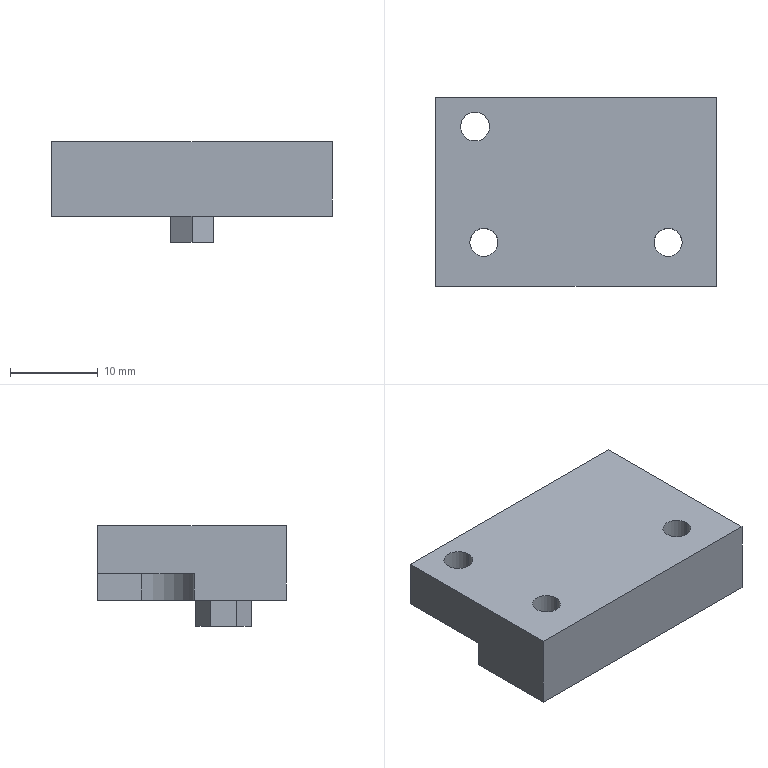Part | NX | 1 solid | 33 faces | box 32 x 21.5 x 11.5 mm | volume 4996 mm3 | plane 18 | cylinder 13 | cone 2 | commonest cylinder face diameters 3.2 x4 6 x4 3.3 x2 4.2 x2 12 x1
STEP:
#1=CARTESIAN_POINT('',(21.,4.,45.3));
#2=VERTEX_POINT('',#1);
#3=CARTESIAN_POINT('',(27.,4.,45.3));
#4=VERTEX_POINT('',#3);
#5=CARTESIAN_POINT('',(24.,4.,45.3));
#6=DIRECTION('',(0.,0.,1.));
#7=DIRECTION('',(-1.,0.,0.));
#8=AXIS2_PLACEMENT_3D('',#5,#6,#7);
#9=CIRCLE('',#8,3.);
#10=EDGE_CURVE('',#2,#4,#9,.T.);
#11=ORIENTED_EDGE('',*,*,#10,.F.);
#12=CARTESIAN_POINT('',(24.,4.,45.3));
#13=DIRECTION('',(0.,0.,1.));
#14=DIRECTION('',(-1.,0.,0.));
#15=AXIS2_PLACEMENT_3D('',#12,#13,#14);
#16=CIRCLE('',#15,3.);
#17=EDGE_CURVE('',#4,#2,#16,.T.);
#18=ORIENTED_EDGE('',*,*,#17,.F.);
#19=EDGE_LOOP('',(#11,#18));
#20=FACE_BOUND('',#19,.T.);
#21=CARTESIAN_POINT('',(25.6,4.,45.3));
#22=VERTEX_POINT('',#21);
#23=CARTESIAN_POINT('',(22.4,4.,45.3));
#24=VERTEX_POINT('',#23);
#25=CARTESIAN_POINT('',(24.,4.,45.3));
#26=DIRECTION('',(0.,0.,1.));
#27=DIRECTION('',(-1.,0.,0.));
#28=AXIS2_PLACEMENT_3D('',#25,#26,#27);
#29=CIRCLE('',#28,1.6);
#30=EDGE_CURVE('',#22,#24,#29,.T.);
#31=ORIENTED_EDGE('',*,*,#30,.T.);
#32=CARTESIAN_POINT('',(24.,4.,45.3));
#33=DIRECTION('',(0.,0.,1.));
#34=DIRECTION('',(-1.,0.,0.));
#35=AXIS2_PLACEMENT_3D('',#32,#33,#34);
#36=CIRCLE('',#35,1.6);
#37=EDGE_CURVE('',#24,#22,#36,.T.);
#38=ORIENTED_EDGE('',*,*,#37,.T.);
#39=EDGE_LOOP('',(#31,#38));
#40=FACE_BOUND('',#39,.T.);
#41=CARTESIAN_POINT('',(24.,4.,45.3));
#42=DIRECTION('',(0.,0.,1.));
#43=DIRECTION('',(1.,0.,0.));
#44=AXIS2_PLACEMENT_3D('',#41,#42,#43);
#45=PLANE('',#44);
#46=ADVANCED_FACE('',(#20,#40),#45,.F.);
#47=CARTESIAN_POINT('',(-2.5,-1.,50.5));
#48=VERTEX_POINT('',#47);
#49=CARTESIAN_POINT('',(-2.5,-1.,42.));
#50=VERTEX_POINT('',#49);
#51=CARTESIAN_POINT('',(-2.5,-1.,0.));
#52=DIRECTION('',(0.,0.,-1.));
#53=VECTOR('',#52,1000.);
#54=LINE('',#51,#53);
#55=EDGE_CURVE('',#48,#50,#54,.T.);
#56=ORIENTED_EDGE('',*,*,#55,.T.);
#57=CARTESIAN_POINT('',(29.5,-1.,42.));
#58=VERTEX_POINT('',#57);
#59=CARTESIAN_POINT('',(0.,-1.,42.));
#60=DIRECTION('',(1.,0.,0.));
#61=VECTOR('',#60,1000.);
#62=LINE('',#59,#61);
#63=EDGE_CURVE('',#50,#58,#62,.T.);
#64=ORIENTED_EDGE('',*,*,#63,.T.);
#65=CARTESIAN_POINT('',(29.5,-1.,50.5));
#66=VERTEX_POINT('',#65);
#67=CARTESIAN_POINT('',(29.5,-1.,0.));
#68=DIRECTION('',(0.,0.,-1.));
#69=VECTOR('',#68,1000.);
#70=LINE('',#67,#69);
#71=EDGE_CURVE('',#66,#58,#70,.T.);
#72=ORIENTED_EDGE('',*,*,#71,.F.);
#73=CARTESIAN_POINT('',(0.,-1.,50.5));
#74=DIRECTION('',(1.,0.,0.));
#75=VECTOR('',#74,1000.);
#76=LINE('',#73,#75);
#77=EDGE_CURVE('',#48,#66,#76,.T.);
#78=ORIENTED_EDGE('',*,*,#77,.F.);
#79=EDGE_LOOP('',(#56,#64,#72,#78));
#80=FACE_BOUND('',#79,.T.);
#81=CARTESIAN_POINT('',(0.,-1.,50.5));
#82=DIRECTION('',(0.,1.,0.));
#83=DIRECTION('',(1.,0.,0.));
#84=AXIS2_PLACEMENT_3D('',#81,#82,#83);
#85=PLANE('',#84);
#86=ADVANCED_FACE('',(#80),#85,.F.);
#87=CARTESIAN_POINT('',(-2.5,9.5,42.));
#88=VERTEX_POINT('',#87);
#89=CARTESIAN_POINT('',(-2.5,0.,42.));
#90=DIRECTION('',(0.,-1.,0.));
#91=VECTOR('',#90,1000.);
#92=LINE('',#89,#91);
#93=EDGE_CURVE('',#88,#50,#92,.T.);
#94=ORIENTED_EDGE('',*,*,#93,.T.);
#95=ORIENTED_EDGE('',*,*,#55,.F.);
#96=CARTESIAN_POINT('',(-2.5,20.5,50.5));
#97=VERTEX_POINT('',#96);
#98=CARTESIAN_POINT('',(-2.5,0.,50.5));
#99=DIRECTION('',(0.,-1.,0.));
#100=VECTOR('',#99,1000.);
#101=LINE('',#98,#100);
#102=EDGE_CURVE('',#97,#48,#101,.T.);
#103=ORIENTED_EDGE('',*,*,#102,.F.);
#104=CARTESIAN_POINT('',(-2.5,20.5,45.));
#105=VERTEX_POINT('',#104);
#106=CARTESIAN_POINT('',(-2.5,20.5,0.));
#107=DIRECTION('',(0.,0.,1.));
#108=VECTOR('',#107,1000.);
#109=LINE('',#106,#108);
#110=EDGE_CURVE('',#105,#97,#109,.T.);
#111=ORIENTED_EDGE('',*,*,#110,.F.);
#112=CARTESIAN_POINT('',(-2.5,9.5,45.));
#113=VERTEX_POINT('',#112);
#114=CARTESIAN_POINT('',(-2.5,0.,45.));
#115=DIRECTION('',(0.,-1.,0.));
#116=VECTOR('',#115,1000.);
#117=LINE('',#114,#116);
#118=EDGE_CURVE('',#105,#113,#117,.T.);
#119=ORIENTED_EDGE('',*,*,#118,.T.);
#120=CARTESIAN_POINT('',(-2.5,9.5,0.));
#121=DIRECTION('',(0.,0.,-1.));
#122=VECTOR('',#121,1000.);
#123=LINE('',#120,#122);
#124=EDGE_CURVE('',#113,#88,#123,.T.);
#125=ORIENTED_EDGE('',*,*,#124,.T.);
#126=EDGE_LOOP('',(#94,#95,#103,#111,#119,#125));
#127=FACE_BOUND('',#126,.T.);
#128=CARTESIAN_POINT('',(-2.5,19.5,50.5));
#129=DIRECTION('',(1.,0.,0.));
#130=DIRECTION('',(0.,1.,0.));
#131=AXIS2_PLACEMENT_3D('',#128,#129,#130);
#132=PLANE('',#131);
#133=ADVANCED_FACE('',(#127),#132,.F.);
#134=ORIENTED_EDGE('',*,*,#124,.F.);
#135=CARTESIAN_POINT('',(4.,9.5,45.));
#136=VERTEX_POINT('',#135);
#137=CARTESIAN_POINT('',(0.,9.5,45.));
#138=DIRECTION('',(1.,0.,0.));
#139=VECTOR('',#138,1000.);
#140=LINE('',#137,#139);
#141=EDGE_CURVE('',#113,#136,#140,.T.);
#142=ORIENTED_EDGE('',*,*,#141,.T.);
#143=CARTESIAN_POINT('',(4.,9.5,42.));
#144=VERTEX_POINT('',#143);
#145=CARTESIAN_POINT('',(4.,9.5,42.));
#146=DIRECTION('',(0.,0.,-1.));
#147=VECTOR('',#146,1000.);
#148=LINE('',#145,#147);
#149=EDGE_CURVE('',#136,#144,#148,.T.);
#150=ORIENTED_EDGE('',*,*,#149,.T.);
#151=CARTESIAN_POINT('',(0.,9.5,42.));
#152=DIRECTION('',(1.,0.,0.));
#153=VECTOR('',#152,1000.);
#154=LINE('',#151,#153);
#155=EDGE_CURVE('',#88,#144,#154,.T.);
#156=ORIENTED_EDGE('',*,*,#155,.F.);
#157=EDGE_LOOP('',(#134,#142,#150,#156));
#158=FACE_BOUND('',#157,.T.);
#159=CARTESIAN_POINT('',(-2.,9.5,42.));
#160=DIRECTION('',(0.,1.,0.));
#161=DIRECTION('',(1.,0.,0.));
#162=AXIS2_PLACEMENT_3D('',#159,#160,#161);
#163=PLANE('',#162);
#164=ADVANCED_FACE('',(#158),#163,.T.);
#165=CARTESIAN_POINT('',(10.,20.5,45.));
#166=VERTEX_POINT('',#165);
#167=CARTESIAN_POINT('',(0.,20.5,45.));
#168=DIRECTION('',(-1.,0.,0.));
#169=VECTOR('',#168,1000.);
#170=LINE('',#167,#169);
#171=EDGE_CURVE('',#166,#105,#170,.T.);
#172=ORIENTED_EDGE('',*,*,#171,.F.);
#173=CARTESIAN_POINT('',(10.,15.5,45.));
#174=VERTEX_POINT('',#173);
#175=CARTESIAN_POINT('',(10.,0.,45.));
#176=DIRECTION('',(0.,1.,0.));
#177=VECTOR('',#176,1000.);
#178=LINE('',#175,#177);
#179=EDGE_CURVE('',#174,#166,#178,.T.);
#180=ORIENTED_EDGE('',*,*,#179,.F.);
#181=CARTESIAN_POINT('',(4.,15.5,45.));
#182=DIRECTION('',(0.,0.,1.));
#183=DIRECTION('',(1.,0.,0.));
#184=AXIS2_PLACEMENT_3D('',#181,#182,#183);
#185=CIRCLE('',#184,6.);
#186=EDGE_CURVE('',#136,#174,#185,.T.);
#187=ORIENTED_EDGE('',*,*,#186,.F.);
#188=ORIENTED_EDGE('',*,*,#141,.F.);
#189=ORIENTED_EDGE('',*,*,#118,.F.);
#190=EDGE_LOOP('',(#172,#180,#187,#188,#189));
#191=FACE_BOUND('',#190,.T.);
#192=CARTESIAN_POINT('',(0.35,17.2,45.));
#193=VERTEX_POINT('',#192);
#194=CARTESIAN_POINT('',(3.65,17.2,45.));
#195=VERTEX_POINT('',#194);
#196=CARTESIAN_POINT('',(2.,17.2,45.));
#197=DIRECTION('',(0.,0.,1.));
#198=DIRECTION('',(1.,0.,0.));
#199=AXIS2_PLACEMENT_3D('',#196,#197,#198);
#200=CIRCLE('',#199,1.65);
#201=EDGE_CURVE('',#193,#195,#200,.T.);
#202=ORIENTED_EDGE('',*,*,#201,.T.);
#203=CARTESIAN_POINT('',(2.,17.2,45.));
#204=DIRECTION('',(0.,0.,1.));
#205=DIRECTION('',(1.,0.,0.));
#206=AXIS2_PLACEMENT_3D('',#203,#204,#205);
#207=CIRCLE('',#206,1.65);
#208=EDGE_CURVE('',#195,#193,#207,.T.);
#209=ORIENTED_EDGE('',*,*,#208,.T.);
#210=EDGE_LOOP('',(#202,#209));
#211=FACE_BOUND('',#210,.T.);
#212=CARTESIAN_POINT('',(0.,0.,45.));
#213=DIRECTION('',(0.,0.,1.));
#214=DIRECTION('',(1.,0.,0.));
#215=AXIS2_PLACEMENT_3D('',#212,#213,#214);
#216=PLANE('',#215);
#217=ADVANCED_FACE('',(#191,#211),#216,.F.);
#218=ORIENTED_EDGE('',*,*,#149,.F.);
#219=ORIENTED_EDGE('',*,*,#186,.T.);
#220=CARTESIAN_POINT('',(10.,15.5,42.));
#221=VERTEX_POINT('',#220);
#222=CARTESIAN_POINT('',(10.,15.5,42.));
#223=DIRECTION('',(0.,0.,-1.));
#224=VECTOR('',#223,1000.);
#225=LINE('',#222,#224);
#226=EDGE_CURVE('',#174,#221,#225,.T.);
#227=ORIENTED_EDGE('',*,*,#226,.T.);
#228=CARTESIAN_POINT('',(4.,15.5,42.));
#229=DIRECTION('',(0.,0.,1.));
#230=DIRECTION('',(1.,0.,0.));
#231=AXIS2_PLACEMENT_3D('',#228,#229,#230);
#232=CIRCLE('',#231,6.);
#233=EDGE_CURVE('',#144,#221,#232,.T.);
#234=ORIENTED_EDGE('',*,*,#233,.F.);
#235=EDGE_LOOP('',(#218,#219,#227,#234));
#236=FACE_BOUND('',#235,.T.);
#237=CARTESIAN_POINT('',(4.,15.5,42.));
#238=DIRECTION('',(0.,0.,-1.));
#239=DIRECTION('',(1.,0.,0.));
#240=AXIS2_PLACEMENT_3D('',#237,#238,#239);
#241=CYLINDRICAL_SURFACE('',#240,6.);
#242=ADVANCED_FACE('',(#236),#241,.F.);
#243=ORIENTED_EDGE('',*,*,#233,.T.);
#244=CARTESIAN_POINT('',(10.,20.5,42.));
#245=VERTEX_POINT('',#244);
#246=CARTESIAN_POINT('',(10.,0.,42.));
#247=DIRECTION('',(0.,1.,0.));
#248=VECTOR('',#247,1000.);
#249=LINE('',#246,#248);
#250=EDGE_CURVE('',#221,#245,#249,.T.);
#251=ORIENTED_EDGE('',*,*,#250,.T.);
#252=CARTESIAN_POINT('',(29.5,20.5,42.));
#253=VERTEX_POINT('',#252);
#254=CARTESIAN_POINT('',(0.,20.5,42.));
#255=DIRECTION('',(-1.,0.,0.));
#256=VECTOR('',#255,1000.);
#257=LINE('',#254,#256);
#258=EDGE_CURVE('',#253,#245,#257,.T.);
#259=ORIENTED_EDGE('',*,*,#258,.F.);
#260=CARTESIAN_POINT('',(29.5,0.,42.));
#261=DIRECTION('',(0.,1.,0.));
#262=VECTOR('',#261,1000.);
#263=LINE('',#260,#262);
#264=EDGE_CURVE('',#58,#253,#263,.T.);
#265=ORIENTED_EDGE('',*,*,#264,.F.);
#266=ORIENTED_EDGE('',*,*,#63,.F.);
#267=ORIENTED_EDGE('',*,*,#93,.F.);
#268=ORIENTED_EDGE('',*,*,#155,.T.);
#269=EDGE_LOOP('',(#243,#251,#259,#265,#266,#267,#268));
#270=FACE_BOUND('',#269,.T.);
#271=CARTESIAN_POINT('',(6.,4.,42.));
#272=VERTEX_POINT('',#271);
#273=CARTESIAN_POINT('',(0.,4.,42.));
#274=VERTEX_POINT('',#273);
#275=CARTESIAN_POINT('',(3.,4.,42.));
#276=DIRECTION('',(0.,0.,1.));
#277=DIRECTION('',(-1.,0.,0.));
#278=AXIS2_PLACEMENT_3D('',#275,#276,#277);
#279=CIRCLE('',#278,3.);
#280=EDGE_CURVE('',#272,#274,#279,.T.);
#281=ORIENTED_EDGE('',*,*,#280,.T.);
#282=CARTESIAN_POINT('',(3.,4.,42.));
#283=DIRECTION('',(0.,0.,1.));
#284=DIRECTION('',(-1.,0.,0.));
#285=AXIS2_PLACEMENT_3D('',#282,#283,#284);
#286=CIRCLE('',#285,3.);
#287=EDGE_CURVE('',#274,#272,#286,.T.);
#288=ORIENTED_EDGE('',*,*,#287,.T.);
#289=EDGE_LOOP('',(#281,#288));
#290=FACE_BOUND('',#289,.T.);
#291=CARTESIAN_POINT('',(11.,7.658,42.));
#292=VERTEX_POINT('',#291);
#293=CARTESIAN_POINT('',(11.,4.658,42.));
#294=VERTEX_POINT('',#293);
#295=CARTESIAN_POINT('',(11.,0.,42.));
#296=DIRECTION('',(0.,-1.,0.));
#297=VECTOR('',#296,1000.);
#298=LINE('',#295,#297);
#299=EDGE_CURVE('',#292,#294,#298,.T.);
#300=ORIENTED_EDGE('',*,*,#299,.T.);
#301=CARTESIAN_POINT('',(13.5,3.,42.));
#302=VERTEX_POINT('',#301);
#303=CARTESIAN_POINT('',(0.,11.955,42.));
#304=DIRECTION('',(0.8333,-0.5528,0.));
#305=VECTOR('',#304,1000.);
#306=LINE('',#303,#305);
#307=EDGE_CURVE('',#294,#302,#306,.T.);
#308=ORIENTED_EDGE('',*,*,#307,.T.);
#309=CARTESIAN_POINT('',(16.,4.658,42.));
#310=VERTEX_POINT('',#309);
#311=CARTESIAN_POINT('',(0.,-5.955,42.));
#312=DIRECTION('',(0.8333,0.5528,0.));
#313=VECTOR('',#312,1000.);
#314=LINE('',#311,#313);
#315=EDGE_CURVE('',#302,#310,#314,.T.);
#316=ORIENTED_EDGE('',*,*,#315,.T.);
#317=CARTESIAN_POINT('',(16.,7.658,42.));
#318=VERTEX_POINT('',#317);
#319=CARTESIAN_POINT('',(16.,0.,42.));
#320=DIRECTION('',(0.,1.,0.));
#321=VECTOR('',#320,1000.);
#322=LINE('',#319,#321);
#323=EDGE_CURVE('',#310,#318,#322,.T.);
#324=ORIENTED_EDGE('',*,*,#323,.T.);
#325=CARTESIAN_POINT('',(13.5,9.317,42.));
#326=VERTEX_POINT('',#325);
#327=CARTESIAN_POINT('',(0.,18.272,42.));
#328=DIRECTION('',(-0.8333,0.5528,0.));
#329=VECTOR('',#328,1000.);
#330=LINE('',#327,#329);
#331=EDGE_CURVE('',#318,#326,#330,.T.);
#332=ORIENTED_EDGE('',*,*,#331,.T.);
#333=CARTESIAN_POINT('',(0.,0.3617,42.));
#334=DIRECTION('',(-0.8333,-0.5528,0.));
#335=VECTOR('',#334,1000.);
#336=LINE('',#333,#335);
#337=EDGE_CURVE('',#326,#292,#336,.T.);
#338=ORIENTED_EDGE('',*,*,#337,.T.);
#339=EDGE_LOOP('',(#300,#308,#316,#324,#332,#338));
#340=FACE_BOUND('',#339,.T.);
#341=CARTESIAN_POINT('',(27.,4.,42.));
#342=VERTEX_POINT('',#341);
#343=CARTESIAN_POINT('',(21.,4.,42.));
#344=VERTEX_POINT('',#343);
#345=CARTESIAN_POINT('',(24.,4.,42.));
#346=DIRECTION('',(0.,0.,1.));
#347=DIRECTION('',(-1.,0.,0.));
#348=AXIS2_PLACEMENT_3D('',#345,#346,#347);
#349=CIRCLE('',#348,3.);
#350=EDGE_CURVE('',#342,#344,#349,.T.);
#351=ORIENTED_EDGE('',*,*,#350,.T.);
#352=CARTESIAN_POINT('',(24.,4.,42.));
#353=DIRECTION('',(0.,0.,1.));
#354=DIRECTION('',(-1.,0.,0.));
#355=AXIS2_PLACEMENT_3D('',#352,#353,#354);
#356=CIRCLE('',#355,3.);
#357=EDGE_CURVE('',#344,#342,#356,.T.);
#358=ORIENTED_EDGE('',*,*,#357,.T.);
#359=EDGE_LOOP('',(#351,#358));
#360=FACE_BOUND('',#359,.T.);
#361=CARTESIAN_POINT('',(0.,0.,42.));
#362=DIRECTION('',(0.,0.,1.));
#363=DIRECTION('',(1.,0.,0.));
#364=AXIS2_PLACEMENT_3D('',#361,#362,#363);
#365=PLANE('',#364);
#366=ADVANCED_FACE('',(#270,#290,#340,#360),#365,.F.);
#367=ORIENTED_EDGE('',*,*,#171,.T.);
#368=ORIENTED_EDGE('',*,*,#110,.T.);
#369=CARTESIAN_POINT('',(29.5,20.5,50.5));
#370=VERTEX_POINT('',#369);
#371=CARTESIAN_POINT('',(0.,20.5,50.5));
#372=DIRECTION('',(-1.,0.,0.));
#373=VECTOR('',#372,1000.);
#374=LINE('',#371,#373);
#375=EDGE_CURVE('',#370,#97,#374,.T.);
#376=ORIENTED_EDGE('',*,*,#375,.F.);
#377=CARTESIAN_POINT('',(29.5,20.5,0.));
#378=DIRECTION('',(0.,0.,-1.));
#379=VECTOR('',#378,1000.);
#380=LINE('',#377,#379);
#381=EDGE_CURVE('',#370,#253,#380,.T.);
#382=ORIENTED_EDGE('',*,*,#381,.T.);
#383=ORIENTED_EDGE('',*,*,#258,.T.);
#384=CARTESIAN_POINT('',(10.,20.5,0.));
#385=DIRECTION('',(0.,0.,-1.));
#386=VECTOR('',#385,1000.);
#387=LINE('',#384,#386);
#388=EDGE_CURVE('',#166,#245,#387,.T.);
#389=ORIENTED_EDGE('',*,*,#388,.F.);
#390=EDGE_LOOP('',(#367,#368,#376,#382,#383,#389));
#391=FACE_BOUND('',#390,.T.);
#392=CARTESIAN_POINT('',(27.,20.5,50.5));
#393=DIRECTION('',(0.,-1.,0.));
#394=DIRECTION('',(0.,0.,-1.));
#395=AXIS2_PLACEMENT_3D('',#392,#393,#394);
#396=PLANE('',#395);
#397=ADVANCED_FACE('',(#391),#396,.F.);
#398=ORIENTED_EDGE('',*,*,#226,.F.);
#399=ORIENTED_EDGE('',*,*,#179,.T.);
#400=ORIENTED_EDGE('',*,*,#388,.T.);
#401=ORIENTED_EDGE('',*,*,#250,.F.);
#402=EDGE_LOOP('',(#398,#399,#400,#401));
#403=FACE_BOUND('',#402,.T.);
#404=CARTESIAN_POINT('',(10.,15.5,42.));
#405=DIRECTION('',(-1.,0.,0.));
#406=DIRECTION('',(0.,0.,1.));
#407=AXIS2_PLACEMENT_3D('',#404,#405,#406);
#408=PLANE('',#407);
#409=ADVANCED_FACE('',(#403),#408,.T.);
#410=CARTESIAN_POINT('',(29.5,0.,50.5));
#411=DIRECTION('',(0.,1.,0.));
#412=VECTOR('',#411,1000.);
#413=LINE('',#410,#412);
#414=EDGE_CURVE('',#66,#370,#413,.T.);
#415=ORIENTED_EDGE('',*,*,#414,.T.);
#416=ORIENTED_EDGE('',*,*,#375,.T.);
#417=ORIENTED_EDGE('',*,*,#102,.T.);
#418=ORIENTED_EDGE('',*,*,#77,.T.);
#419=EDGE_LOOP('',(#415,#416,#417,#418));
#420=FACE_BOUND('',#419,.T.);
#421=CARTESIAN_POINT('',(1.4,4.,50.5));
#422=VERTEX_POINT('',#421);
#423=CARTESIAN_POINT('',(4.6,4.,50.5));
#424=VERTEX_POINT('',#423);
#425=CARTESIAN_POINT('',(3.,4.,50.5));
#426=DIRECTION('',(0.,0.,1.));
#427=DIRECTION('',(-1.,0.,0.));
#428=AXIS2_PLACEMENT_3D('',#425,#426,#427);
#429=CIRCLE('',#428,1.6);
#430=EDGE_CURVE('',#422,#424,#429,.T.);
#431=ORIENTED_EDGE('',*,*,#430,.F.);
#432=CARTESIAN_POINT('',(3.,4.,50.5));
#433=DIRECTION('',(0.,0.,1.));
#434=DIRECTION('',(-1.,0.,0.));
#435=AXIS2_PLACEMENT_3D('',#432,#433,#434);
#436=CIRCLE('',#435,1.6);
#437=EDGE_CURVE('',#424,#422,#436,.T.);
#438=ORIENTED_EDGE('',*,*,#437,.F.);
#439=EDGE_LOOP('',(#431,#438));
#440=FACE_BOUND('',#439,.T.);
#441=CARTESIAN_POINT('',(3.65,17.2,50.5));
#442=VERTEX_POINT('',#441);
#443=CARTESIAN_POINT('',(0.35,17.2,50.5));
#444=VERTEX_POINT('',#443);
#445=CARTESIAN_POINT('',(2.,17.2,50.5));
#446=DIRECTION('',(0.,0.,1.));
#447=DIRECTION('',(1.,0.,0.));
#448=AXIS2_PLACEMENT_3D('',#445,#446,#447);
#449=CIRCLE('',#448,1.65);
#450=EDGE_CURVE('',#442,#444,#449,.T.);
#451=ORIENTED_EDGE('',*,*,#450,.F.);
#452=CARTESIAN_POINT('',(2.,17.2,50.5));
#453=DIRECTION('',(0.,0.,1.));
#454=DIRECTION('',(1.,0.,0.));
#455=AXIS2_PLACEMENT_3D('',#452,#453,#454);
#456=CIRCLE('',#455,1.65);
#457=EDGE_CURVE('',#444,#442,#456,.T.);
#458=ORIENTED_EDGE('',*,*,#457,.F.);
#459=EDGE_LOOP('',(#451,#458));
#460=FACE_BOUND('',#459,.T.);
#461=CARTESIAN_POINT('',(22.4,4.,50.5));
#462=VERTEX_POINT('',#461);
#463=CARTESIAN_POINT('',(25.6,4.,50.5));
#464=VERTEX_POINT('',#463);
#465=CARTESIAN_POINT('',(24.,4.,50.5));
#466=DIRECTION('',(0.,0.,1.));
#467=DIRECTION('',(-1.,0.,0.));
#468=AXIS2_PLACEMENT_3D('',#465,#466,#467);
#469=CIRCLE('',#468,1.6);
#470=EDGE_CURVE('',#462,#464,#469,.T.);
#471=ORIENTED_EDGE('',*,*,#470,.F.);
#472=CARTESIAN_POINT('',(24.,4.,50.5));
#473=DIRECTION('',(0.,0.,1.));
#474=DIRECTION('',(-1.,0.,0.));
#475=AXIS2_PLACEMENT_3D('',#472,#473,#474);
#476=CIRCLE('',#475,1.6);
#477=EDGE_CURVE('',#464,#462,#476,.T.);
#478=ORIENTED_EDGE('',*,*,#477,.F.);
#479=EDGE_LOOP('',(#471,#478));
#480=FACE_BOUND('',#479,.T.);
#481=CARTESIAN_POINT('',(0.,0.,50.5));
#482=DIRECTION('',(0.,0.,1.));
#483=DIRECTION('',(1.,0.,0.));
#484=AXIS2_PLACEMENT_3D('',#481,#482,#483);
#485=PLANE('',#484);
#486=ADVANCED_FACE('',(#420,#440,#460,#480),#485,.T.);
#487=CARTESIAN_POINT('',(29.5,7.9,46.5));
#488=VERTEX_POINT('',#487);
#489=CARTESIAN_POINT('',(29.5,12.1,46.5));
#490=VERTEX_POINT('',#489);
#491=CARTESIAN_POINT('',(29.5,10.,46.5));
#492=DIRECTION('',(-1.,0.,0.));
#493=DIRECTION('',(0.,-1.,0.));
#494=AXIS2_PLACEMENT_3D('',#491,#492,#493);
#495=CIRCLE('',#494,2.1);
#496=EDGE_CURVE('',#488,#490,#495,.T.);
#497=ORIENTED_EDGE('',*,*,#496,.F.);
#498=CARTESIAN_POINT('',(14.4,7.9,46.5));
#499=VERTEX_POINT('',#498);
#500=CARTESIAN_POINT('',(12.445,7.9,46.5));
#501=DIRECTION('',(1.,0.,0.));
#502=VECTOR('',#501,1000.);
#503=LINE('',#500,#502);
#504=EDGE_CURVE('',#488,#499,#503,.F.);
#505=ORIENTED_EDGE('',*,*,#504,.T.);
#506=CARTESIAN_POINT('',(14.4,12.1,46.5));
#507=VERTEX_POINT('',#506);
#508=CARTESIAN_POINT('',(14.4,10.,46.5));
#509=DIRECTION('',(-1.,0.,0.));
#510=DIRECTION('',(0.,-1.,0.));
#511=AXIS2_PLACEMENT_3D('',#508,#509,#510);
#512=CIRCLE('',#511,2.1);
#513=EDGE_CURVE('',#499,#507,#512,.T.);
#514=ORIENTED_EDGE('',*,*,#513,.T.);
#515=CARTESIAN_POINT('',(12.445,12.1,46.5));
#516=DIRECTION('',(1.,0.,0.));
#517=VECTOR('',#516,1000.);
#518=LINE('',#515,#517);
#519=EDGE_CURVE('',#490,#507,#518,.F.);
#520=ORIENTED_EDGE('',*,*,#519,.F.);
#521=EDGE_LOOP('',(#497,#505,#514,#520));
#522=FACE_BOUND('',#521,.T.);
#523=CARTESIAN_POINT('',(12.445,10.,46.5));
#524=DIRECTION('',(1.,0.,0.));
#525=DIRECTION('',(0.,-1.,0.));
#526=AXIS2_PLACEMENT_3D('',#523,#524,#525);
#527=CYLINDRICAL_SURFACE('',#526,2.1);
#528=ADVANCED_FACE('',(#522),#527,.F.);
#529=CARTESIAN_POINT('',(11.,7.658,39.));
#530=VERTEX_POINT('',#529);
#531=CARTESIAN_POINT('',(11.,7.658,0.));
#532=DIRECTION('',(0.,0.,1.));
#533=VECTOR('',#532,1000.);
#534=LINE('',#531,#533);
#535=EDGE_CURVE('',#530,#292,#534,.T.);
#536=ORIENTED_EDGE('',*,*,#535,.F.);
#537=CARTESIAN_POINT('',(11.,4.658,39.));
#538=VERTEX_POINT('',#537);
#539=CARTESIAN_POINT('',(11.,0.,39.));
#540=DIRECTION('',(0.,-1.,0.));
#541=VECTOR('',#540,1000.);
#542=LINE('',#539,#541);
#543=EDGE_CURVE('',#530,#538,#542,.T.);
#544=ORIENTED_EDGE('',*,*,#543,.T.);
#545=CARTESIAN_POINT('',(11.,4.658,0.));
#546=DIRECTION('',(0.,0.,1.));
#547=VECTOR('',#546,1000.);
#548=LINE('',#545,#547);
#549=EDGE_CURVE('',#538,#294,#548,.T.);
#550=ORIENTED_EDGE('',*,*,#549,.T.);
#551=ORIENTED_EDGE('',*,*,#299,.F.);
#552=EDGE_LOOP('',(#536,#544,#550,#551));
#553=FACE_BOUND('',#552,.T.);
#554=CARTESIAN_POINT('',(11.,7.658,42.));
#555=DIRECTION('',(1.,0.,0.));
#556=DIRECTION('',(0.,1.,0.));
#557=AXIS2_PLACEMENT_3D('',#554,#555,#556);
#558=PLANE('',#557);
#559=ADVANCED_FACE('',(#553),#558,.F.);
#560=CARTESIAN_POINT('',(14.4,10.,46.5));
#561=DIRECTION('',(-1.,0.,0.));
#562=DIRECTION('',(0.,-1.,0.));
#563=AXIS2_PLACEMENT_3D('',#560,#561,#562);
#564=CIRCLE('',#563,2.1);
#565=EDGE_CURVE('',#507,#499,#564,.T.);
#566=ORIENTED_EDGE('',*,*,#565,.F.);
#567=CARTESIAN_POINT('',(13.138,10.,46.5));
#568=VERTEX_POINT('',#567);
#569=CARTESIAN_POINT('',(13.782,11.071,46.5));
#570=DIRECTION('',(0.515,0.8572,0.));
#571=VECTOR('',#570,1000.);
#572=LINE('',#569,#571);
#573=EDGE_CURVE('',#568,#507,#572,.T.);
#574=ORIENTED_EDGE('',*,*,#573,.F.);
#575=CARTESIAN_POINT('',(13.782,8.929,46.5));
#576=DIRECTION('',(0.515,-0.8572,0.));
#577=VECTOR('',#576,1000.);
#578=LINE('',#575,#577);
#579=EDGE_CURVE('',#568,#499,#578,.T.);
#580=ORIENTED_EDGE('',*,*,#579,.T.);
#581=EDGE_LOOP('',(#566,#574,#580));
#582=FACE_BOUND('',#581,.T.);
#583=CARTESIAN_POINT('',(13.782,10.,46.5));
#584=DIRECTION('',(1.,0.,0.));
#585=DIRECTION('',(0.,-1.,0.));
#586=AXIS2_PLACEMENT_3D('',#583,#584,#585);
#587=CONICAL_SURFACE('',#586,1.071,1.03);
#588=ADVANCED_FACE('',(#582),#587,.F.);
#589=CARTESIAN_POINT('',(16.,7.658,39.));
#590=VERTEX_POINT('',#589);
#591=CARTESIAN_POINT('',(13.5,9.317,39.));
#592=VERTEX_POINT('',#591);
#593=CARTESIAN_POINT('',(0.,18.272,39.));
#594=DIRECTION('',(-0.8333,0.5528,0.));
#595=VECTOR('',#594,1000.);
#596=LINE('',#593,#595);
#597=EDGE_CURVE('',#590,#592,#596,.T.);
#598=ORIENTED_EDGE('',*,*,#597,.F.);
#599=CARTESIAN_POINT('',(16.,4.658,39.));
#600=VERTEX_POINT('',#599);
#601=CARTESIAN_POINT('',(16.,0.,39.));
#602=DIRECTION('',(0.,1.,0.));
#603=VECTOR('',#602,1000.);
#604=LINE('',#601,#603);
#605=EDGE_CURVE('',#600,#590,#604,.T.);
#606=ORIENTED_EDGE('',*,*,#605,.F.);
#607=CARTESIAN_POINT('',(13.5,3.,39.));
#608=VERTEX_POINT('',#607);
#609=CARTESIAN_POINT('',(0.,-5.955,39.));
#610=DIRECTION('',(0.8333,0.5528,0.));
#611=VECTOR('',#610,1000.);
#612=LINE('',#609,#611);
#613=EDGE_CURVE('',#608,#600,#612,.T.);
#614=ORIENTED_EDGE('',*,*,#613,.F.);
#615=CARTESIAN_POINT('',(0.,11.955,39.));
#616=DIRECTION('',(-0.8333,0.5528,0.));
#617=VECTOR('',#616,1000.);
#618=LINE('',#615,#617);
#619=EDGE_CURVE('',#608,#538,#618,.T.);
#620=ORIENTED_EDGE('',*,*,#619,.T.);
#621=ORIENTED_EDGE('',*,*,#543,.F.);
#622=CARTESIAN_POINT('',(0.,0.3617,39.));
#623=DIRECTION('',(-0.8333,-0.5528,0.));
#624=VECTOR('',#623,1000.);
#625=LINE('',#622,#624);
#626=EDGE_CURVE('',#592,#530,#625,.T.);
#627=ORIENTED_EDGE('',*,*,#626,.F.);
#628=EDGE_LOOP('',(#598,#606,#614,#620,#621,#627));
#629=FACE_BOUND('',#628,.T.);
#630=CARTESIAN_POINT('',(0.,0.,39.));
#631=DIRECTION('',(0.,0.,1.));
#632=DIRECTION('',(1.,0.,0.));
#633=AXIS2_PLACEMENT_3D('',#630,#631,#632);
#634=PLANE('',#633);
#635=ADVANCED_FACE('',(#629),#634,.F.);
#636=ORIENTED_EDGE('',*,*,#201,.F.);
#637=CARTESIAN_POINT('',(0.35,17.2,52.955));
#638=DIRECTION('',(0.,0.,-1.));
#639=VECTOR('',#638,1000.);
#640=LINE('',#637,#639);
#641=EDGE_CURVE('',#193,#444,#640,.F.);
#642=ORIENTED_EDGE('',*,*,#641,.T.);
#643=ORIENTED_EDGE('',*,*,#457,.T.);
#644=CARTESIAN_POINT('',(3.65,17.2,52.955));
#645=DIRECTION('',(0.,0.,-1.));
#646=VECTOR('',#645,1000.);
#647=LINE('',#644,#646);
#648=EDGE_CURVE('',#195,#442,#647,.F.);
#649=ORIENTED_EDGE('',*,*,#648,.F.);
#650=EDGE_LOOP('',(#636,#642,#643,#649));
#651=FACE_BOUND('',#650,.T.);
#652=CARTESIAN_POINT('',(2.,17.2,52.955));
#653=DIRECTION('',(0.,0.,-1.));
#654=DIRECTION('',(1.,0.,0.));
#655=AXIS2_PLACEMENT_3D('',#652,#653,#654);
#656=CYLINDRICAL_SURFACE('',#655,1.65);
#657=ADVANCED_FACE('',(#651),#656,.F.);
#658=CARTESIAN_POINT('',(13.5,9.317,0.));
#659=DIRECTION('',(0.,0.,1.));
#660=VECTOR('',#659,1000.);
#661=LINE('',#658,#660);
#662=EDGE_CURVE('',#592,#326,#661,.T.);
#663=ORIENTED_EDGE('',*,*,#662,.F.);
#664=ORIENTED_EDGE('',*,*,#626,.T.);
#665=ORIENTED_EDGE('',*,*,#535,.T.);
#666=ORIENTED_EDGE('',*,*,#337,.F.);
#667=EDGE_LOOP('',(#663,#664,#665,#666));
#668=FACE_BOUND('',#667,.T.);
#669=CARTESIAN_POINT('',(13.5,9.317,42.));
#670=DIRECTION('',(0.5528,-0.8333,0.));
#671=DIRECTION('',(0.,0.,-1.));
#672=AXIS2_PLACEMENT_3D('',#669,#670,#671);
#673=PLANE('',#672);
#674=ADVANCED_FACE('',(#668),#673,.F.);
#675=ORIENTED_EDGE('',*,*,#280,.F.);
#676=CARTESIAN_POINT('',(6.,4.,45.3));
#677=VERTEX_POINT('',#676);
#678=CARTESIAN_POINT('',(6.,4.,51.24));
#679=DIRECTION('',(0.,0.,-1.));
#680=VECTOR('',#679,1000.);
#681=LINE('',#678,#680);
#682=EDGE_CURVE('',#272,#677,#681,.F.);
#683=ORIENTED_EDGE('',*,*,#682,.T.);
#684=CARTESIAN_POINT('',(0.,4.,45.3));
#685=VERTEX_POINT('',#684);
#686=CARTESIAN_POINT('',(3.,4.,45.3));
#687=DIRECTION('',(0.,0.,1.));
#688=DIRECTION('',(-1.,0.,0.));
#689=AXIS2_PLACEMENT_3D('',#686,#687,#688);
#690=CIRCLE('',#689,3.);
#691=EDGE_CURVE('',#677,#685,#690,.T.);
#692=ORIENTED_EDGE('',*,*,#691,.T.);
#693=CARTESIAN_POINT('',(0.,4.,51.24));
#694=DIRECTION('',(0.,0.,-1.));
#695=VECTOR('',#694,1000.);
#696=LINE('',#693,#695);
#697=EDGE_CURVE('',#274,#685,#696,.F.);
#698=ORIENTED_EDGE('',*,*,#697,.F.);
#699=EDGE_LOOP('',(#675,#683,#692,#698));
#700=FACE_BOUND('',#699,.T.);
#701=CARTESIAN_POINT('',(3.,4.,51.24));
#702=DIRECTION('',(0.,0.,-1.));
#703=DIRECTION('',(-1.,0.,0.));
#704=AXIS2_PLACEMENT_3D('',#701,#702,#703);
#705=CYLINDRICAL_SURFACE('',#704,3.);
#706=ADVANCED_FACE('',(#700),#705,.F.);
#707=CARTESIAN_POINT('',(13.5,3.,0.));
#708=DIRECTION('',(0.,0.,-1.));
#709=VECTOR('',#708,1000.);
#710=LINE('',#707,#709);
#711=EDGE_CURVE('',#302,#608,#710,.T.);
#712=ORIENTED_EDGE('',*,*,#711,.T.);
#713=ORIENTED_EDGE('',*,*,#613,.T.);
#714=CARTESIAN_POINT('',(16.,4.658,0.));
#715=DIRECTION('',(0.,0.,-1.));
#716=VECTOR('',#715,1000.);
#717=LINE('',#714,#716);
#718=EDGE_CURVE('',#310,#600,#717,.T.);
#719=ORIENTED_EDGE('',*,*,#718,.F.);
#720=ORIENTED_EDGE('',*,*,#315,.F.);
#721=EDGE_LOOP('',(#712,#713,#719,#720));
#722=FACE_BOUND('',#721,.T.);
#723=CARTESIAN_POINT('',(13.5,3.,42.));
#724=DIRECTION('',(-0.5528,0.8333,0.));
#725=DIRECTION('',(0.,0.,1.));
#726=AXIS2_PLACEMENT_3D('',#723,#724,#725);
#727=PLANE('',#726);
#728=ADVANCED_FACE('',(#722),#727,.F.);
#729=ORIENTED_EDGE('',*,*,#71,.T.);
#730=ORIENTED_EDGE('',*,*,#264,.T.);
#731=ORIENTED_EDGE('',*,*,#381,.F.);
#732=ORIENTED_EDGE('',*,*,#414,.F.);
#733=EDGE_LOOP('',(#729,#730,#731,#732));
#734=FACE_BOUND('',#733,.T.);
#735=ORIENTED_EDGE('',*,*,#496,.T.);
#736=CARTESIAN_POINT('',(29.5,10.,46.5));
#737=DIRECTION('',(-1.,0.,0.));
#738=DIRECTION('',(0.,-1.,0.));
#739=AXIS2_PLACEMENT_3D('',#736,#737,#738);
#740=CIRCLE('',#739,2.1);
#741=EDGE_CURVE('',#490,#488,#740,.T.);
#742=ORIENTED_EDGE('',*,*,#741,.T.);
#743=EDGE_LOOP('',(#735,#742));
#744=FACE_BOUND('',#743,.T.);
#745=CARTESIAN_POINT('',(29.5,0.,50.5));
#746=DIRECTION('',(-1.,0.,0.));
#747=DIRECTION('',(0.,0.,1.));
#748=AXIS2_PLACEMENT_3D('',#745,#746,#747);
#749=PLANE('',#748);
#750=ADVANCED_FACE('',(#734,#744),#749,.F.);
#751=CARTESIAN_POINT('',(1.4,4.,45.3));
#752=VERTEX_POINT('',#751);
#753=CARTESIAN_POINT('',(4.6,4.,45.3));
#754=VERTEX_POINT('',#753);
#755=CARTESIAN_POINT('',(3.,4.,45.3));
#756=DIRECTION('',(0.,0.,1.));
#757=DIRECTION('',(-1.,0.,0.));
#758=AXIS2_PLACEMENT_3D('',#755,#756,#757);
#759=CIRCLE('',#758,1.6);
#760=EDGE_CURVE('',#752,#754,#759,.T.);
#761=ORIENTED_EDGE('',*,*,#760,.F.);
#762=CARTESIAN_POINT('',(1.4,4.,51.74));
#763=DIRECTION('',(0.,0.,-1.));
#764=VECTOR('',#763,1000.);
#765=LINE('',#762,#764);
#766=EDGE_CURVE('',#752,#422,#765,.F.);
#767=ORIENTED_EDGE('',*,*,#766,.T.);
#768=ORIENTED_EDGE('',*,*,#430,.T.);
#769=CARTESIAN_POINT('',(4.6,4.,51.74));
#770=DIRECTION('',(0.,0.,-1.));
#771=VECTOR('',#770,1000.);
#772=LINE('',#769,#771);
#773=EDGE_CURVE('',#754,#424,#772,.F.);
#774=ORIENTED_EDGE('',*,*,#773,.F.);
#775=EDGE_LOOP('',(#761,#767,#768,#774));
#776=FACE_BOUND('',#775,.T.);
#777=CARTESIAN_POINT('',(3.,4.,51.74));
#778=DIRECTION('',(0.,0.,-1.));
#779=DIRECTION('',(-1.,0.,0.));
#780=AXIS2_PLACEMENT_3D('',#777,#778,#779);
#781=CYLINDRICAL_SURFACE('',#780,1.6);
#782=ADVANCED_FACE('',(#776),#781,.F.);
#783=CARTESIAN_POINT('',(16.,7.658,0.));
#784=DIRECTION('',(0.,0.,-1.));
#785=VECTOR('',#784,1000.);
#786=LINE('',#783,#785);
#787=EDGE_CURVE('',#318,#590,#786,.T.);
#788=ORIENTED_EDGE('',*,*,#787,.T.);
#789=ORIENTED_EDGE('',*,*,#597,.T.);
#790=ORIENTED_EDGE('',*,*,#662,.T.);
#791=ORIENTED_EDGE('',*,*,#331,.F.);
#792=EDGE_LOOP('',(#788,#789,#790,#791));
#793=FACE_BOUND('',#792,.T.);
#794=CARTESIAN_POINT('',(16.,7.658,42.));
#795=DIRECTION('',(-0.5528,-0.8333,0.));
#796=DIRECTION('',(-0.8333,0.5528,0.));
#797=AXIS2_PLACEMENT_3D('',#794,#795,#796);
#798=PLANE('',#797);
#799=ADVANCED_FACE('',(#793),#798,.F.);
#800=ORIENTED_EDGE('',*,*,#350,.F.);
#801=CARTESIAN_POINT('',(27.,4.,51.24));
#802=DIRECTION('',(0.,0.,-1.));
#803=VECTOR('',#802,1000.);
#804=LINE('',#801,#803);
#805=EDGE_CURVE('',#4,#342,#804,.T.);
#806=ORIENTED_EDGE('',*,*,#805,.F.);
#807=ORIENTED_EDGE('',*,*,#17,.T.);
#808=CARTESIAN_POINT('',(21.,4.,51.24));
#809=DIRECTION('',(0.,0.,-1.));
#810=VECTOR('',#809,1000.);
#811=LINE('',#808,#810);
#812=EDGE_CURVE('',#2,#344,#811,.T.);
#813=ORIENTED_EDGE('',*,*,#812,.T.);
#814=EDGE_LOOP('',(#800,#806,#807,#813));
#815=FACE_BOUND('',#814,.T.);
#816=CARTESIAN_POINT('',(24.,4.,51.24));
#817=DIRECTION('',(0.,0.,-1.));
#818=DIRECTION('',(-1.,0.,0.));
#819=AXIS2_PLACEMENT_3D('',#816,#817,#818);
#820=CYLINDRICAL_SURFACE('',#819,3.);
#821=ADVANCED_FACE('',(#815),#820,.F.);
#822=ORIENTED_EDGE('',*,*,#718,.T.);
#823=ORIENTED_EDGE('',*,*,#605,.T.);
#824=ORIENTED_EDGE('',*,*,#787,.F.);
#825=ORIENTED_EDGE('',*,*,#323,.F.);
#826=EDGE_LOOP('',(#822,#823,#824,#825));
#827=FACE_BOUND('',#826,.T.);
#828=CARTESIAN_POINT('',(16.,4.658,42.));
#829=DIRECTION('',(-1.,0.,0.));
#830=DIRECTION('',(0.,0.,1.));
#831=AXIS2_PLACEMENT_3D('',#828,#829,#830);
#832=PLANE('',#831);
#833=ADVANCED_FACE('',(#827),#832,.F.);
#834=ORIENTED_EDGE('',*,*,#691,.F.);
#835=CARTESIAN_POINT('',(3.,4.,45.3));
#836=DIRECTION('',(0.,0.,1.));
#837=DIRECTION('',(-1.,0.,0.));
#838=AXIS2_PLACEMENT_3D('',#835,#836,#837);
#839=CIRCLE('',#838,3.);
#840=EDGE_CURVE('',#685,#677,#839,.T.);
#841=ORIENTED_EDGE('',*,*,#840,.F.);
#842=EDGE_LOOP('',(#834,#841));
#843=FACE_BOUND('',#842,.T.);
#844=ORIENTED_EDGE('',*,*,#760,.T.);
#845=CARTESIAN_POINT('',(3.,4.,45.3));
#846=DIRECTION('',(0.,0.,1.));
#847=DIRECTION('',(-1.,0.,0.));
#848=AXIS2_PLACEMENT_3D('',#845,#846,#847);
#849=CIRCLE('',#848,1.6);
#850=EDGE_CURVE('',#754,#752,#849,.T.);
#851=ORIENTED_EDGE('',*,*,#850,.T.);
#852=EDGE_LOOP('',(#844,#851));
#853=FACE_BOUND('',#852,.T.);
#854=CARTESIAN_POINT('',(3.,4.,45.3));
#855=DIRECTION('',(0.,0.,1.));
#856=DIRECTION('',(1.,0.,0.));
#857=AXIS2_PLACEMENT_3D('',#854,#855,#856);
#858=PLANE('',#857);
#859=ADVANCED_FACE('',(#843,#853),#858,.F.);
#860=ORIENTED_EDGE('',*,*,#30,.F.);
#861=CARTESIAN_POINT('',(25.6,4.,51.74));
#862=DIRECTION('',(0.,0.,-1.));
#863=VECTOR('',#862,1000.);
#864=LINE('',#861,#863);
#865=EDGE_CURVE('',#464,#22,#864,.T.);
#866=ORIENTED_EDGE('',*,*,#865,.F.);
#867=ORIENTED_EDGE('',*,*,#477,.T.);
#868=CARTESIAN_POINT('',(22.4,4.,51.74));
#869=DIRECTION('',(0.,0.,-1.));
#870=VECTOR('',#869,1000.);
#871=LINE('',#868,#870);
#872=EDGE_CURVE('',#462,#24,#871,.T.);
#873=ORIENTED_EDGE('',*,*,#872,.T.);
#874=EDGE_LOOP('',(#860,#866,#867,#873));
#875=FACE_BOUND('',#874,.T.);
#876=CARTESIAN_POINT('',(24.,4.,51.74));
#877=DIRECTION('',(0.,0.,-1.));
#878=DIRECTION('',(-1.,0.,0.));
#879=AXIS2_PLACEMENT_3D('',#876,#877,#878);
#880=CYLINDRICAL_SURFACE('',#879,1.6);
#881=ADVANCED_FACE('',(#875),#880,.F.);
#882=ORIENTED_EDGE('',*,*,#549,.F.);
#883=ORIENTED_EDGE('',*,*,#619,.F.);
#884=ORIENTED_EDGE('',*,*,#711,.F.);
#885=ORIENTED_EDGE('',*,*,#307,.F.);
#886=EDGE_LOOP('',(#882,#883,#884,#885));
#887=FACE_BOUND('',#886,.T.);
#888=CARTESIAN_POINT('',(11.,4.658,42.));
#889=DIRECTION('',(0.5528,0.8333,0.));
#890=DIRECTION('',(0.,0.,-1.));
#891=AXIS2_PLACEMENT_3D('',#888,#889,#890);
#892=PLANE('',#891);
#893=ADVANCED_FACE('',(#887),#892,.F.);
#894=ORIENTED_EDGE('',*,*,#573,.T.);
#895=ORIENTED_EDGE('',*,*,#513,.F.);
#896=ORIENTED_EDGE('',*,*,#579,.F.);
#897=EDGE_LOOP('',(#894,#895,#896));
#898=FACE_BOUND('',#897,.T.);
#899=CARTESIAN_POINT('',(13.782,10.,46.5));
#900=DIRECTION('',(1.,0.,0.));
#901=DIRECTION('',(0.,-1.,0.));
#902=AXIS2_PLACEMENT_3D('',#899,#900,#901);
#903=CONICAL_SURFACE('',#902,1.071,1.03);
#904=ADVANCED_FACE('',(#898),#903,.F.);
#905=ORIENTED_EDGE('',*,*,#470,.T.);
#906=ORIENTED_EDGE('',*,*,#865,.T.);
#907=ORIENTED_EDGE('',*,*,#37,.F.);
#908=ORIENTED_EDGE('',*,*,#872,.F.);
#909=EDGE_LOOP('',(#905,#906,#907,#908));
#910=FACE_BOUND('',#909,.T.);
#911=CARTESIAN_POINT('',(24.,4.,51.74));
#912=DIRECTION('',(0.,0.,-1.));
#913=DIRECTION('',(-1.,0.,0.));
#914=AXIS2_PLACEMENT_3D('',#911,#912,#913);
#915=CYLINDRICAL_SURFACE('',#914,1.6);
#916=ADVANCED_FACE('',(#910),#915,.F.);
#917=ORIENTED_EDGE('',*,*,#697,.T.);
#918=ORIENTED_EDGE('',*,*,#840,.T.);
#919=ORIENTED_EDGE('',*,*,#682,.F.);
#920=ORIENTED_EDGE('',*,*,#287,.F.);
#921=EDGE_LOOP('',(#917,#918,#919,#920));
#922=FACE_BOUND('',#921,.T.);
#923=CARTESIAN_POINT('',(3.,4.,51.24));
#924=DIRECTION('',(0.,0.,-1.));
#925=DIRECTION('',(-1.,0.,0.));
#926=AXIS2_PLACEMENT_3D('',#923,#924,#925);
#927=CYLINDRICAL_SURFACE('',#926,3.);
#928=ADVANCED_FACE('',(#922),#927,.F.);
#929=ORIENTED_EDGE('',*,*,#10,.T.);
#930=ORIENTED_EDGE('',*,*,#805,.T.);
#931=ORIENTED_EDGE('',*,*,#357,.F.);
#932=ORIENTED_EDGE('',*,*,#812,.F.);
#933=EDGE_LOOP('',(#929,#930,#931,#932));
#934=FACE_BOUND('',#933,.T.);
#935=CARTESIAN_POINT('',(24.,4.,51.24));
#936=DIRECTION('',(0.,0.,-1.));
#937=DIRECTION('',(-1.,0.,0.));
#938=AXIS2_PLACEMENT_3D('',#935,#936,#937);
#939=CYLINDRICAL_SURFACE('',#938,3.);
#940=ADVANCED_FACE('',(#934),#939,.F.);
#941=ORIENTED_EDGE('',*,*,#450,.T.);
#942=ORIENTED_EDGE('',*,*,#641,.F.);
#943=ORIENTED_EDGE('',*,*,#208,.F.);
#944=ORIENTED_EDGE('',*,*,#648,.T.);
#945=EDGE_LOOP('',(#941,#942,#943,#944));
#946=FACE_BOUND('',#945,.T.);
#947=CARTESIAN_POINT('',(2.,17.2,52.955));
#948=DIRECTION('',(0.,0.,-1.));
#949=DIRECTION('',(1.,0.,0.));
#950=AXIS2_PLACEMENT_3D('',#947,#948,#949);
#951=CYLINDRICAL_SURFACE('',#950,1.65);
#952=ADVANCED_FACE('',(#946),#951,.F.);
#953=ORIENTED_EDGE('',*,*,#766,.F.);
#954=ORIENTED_EDGE('',*,*,#850,.F.);
#955=ORIENTED_EDGE('',*,*,#773,.T.);
#956=ORIENTED_EDGE('',*,*,#437,.T.);
#957=EDGE_LOOP('',(#953,#954,#955,#956));
#958=FACE_BOUND('',#957,.T.);
#959=CARTESIAN_POINT('',(3.,4.,51.74));
#960=DIRECTION('',(0.,0.,-1.));
#961=DIRECTION('',(-1.,0.,0.));
#962=AXIS2_PLACEMENT_3D('',#959,#960,#961);
#963=CYLINDRICAL_SURFACE('',#962,1.6);
#964=ADVANCED_FACE('',(#958),#963,.F.);
#965=ORIENTED_EDGE('',*,*,#565,.T.);
#966=ORIENTED_EDGE('',*,*,#504,.F.);
#967=ORIENTED_EDGE('',*,*,#741,.F.);
#968=ORIENTED_EDGE('',*,*,#519,.T.);
#969=EDGE_LOOP('',(#965,#966,#967,#968));
#970=FACE_BOUND('',#969,.T.);
#971=CARTESIAN_POINT('',(12.445,10.,46.5));
#972=DIRECTION('',(1.,0.,0.));
#973=DIRECTION('',(0.,-1.,0.));
#974=AXIS2_PLACEMENT_3D('',#971,#972,#973);
#975=CYLINDRICAL_SURFACE('',#974,2.1);
#976=ADVANCED_FACE('',(#970),#975,.F.);
#977=CLOSED_SHELL('',(#46,#86,#133,#164,#217,#242,#366,#397,#409,#486,#528,#559,#588,#635,#657,#674,#706,#728,#750,#782,#799,#821,#833,#859,#881,#893,#904,#916,#928,#940,#952,#964,#976));
#978=MANIFOLD_SOLID_BREP('',#977);
#979=(LENGTH_UNIT()NAMED_UNIT(*)SI_UNIT(.MILLI.,.METRE.));
#980=UNCERTAINTY_MEASURE_WITH_UNIT(LENGTH_MEASURE(0.00001),#979,'','');
#981=(NAMED_UNIT(*)PLANE_ANGLE_UNIT()SI_UNIT($,.RADIAN.));
#982=(NAMED_UNIT(*)SI_UNIT($,.STERADIAN.)SOLID_ANGLE_UNIT());
#983=(GEOMETRIC_REPRESENTATION_CONTEXT(3)GLOBAL_UNCERTAINTY_ASSIGNED_CONTEXT((#980))GLOBAL_UNIT_ASSIGNED_CONTEXT((#979,#981,#982))REPRESENTATION_CONTEXT('',''));
#984=ADVANCED_BREP_SHAPE_REPRESENTATION('',(#978),#983);